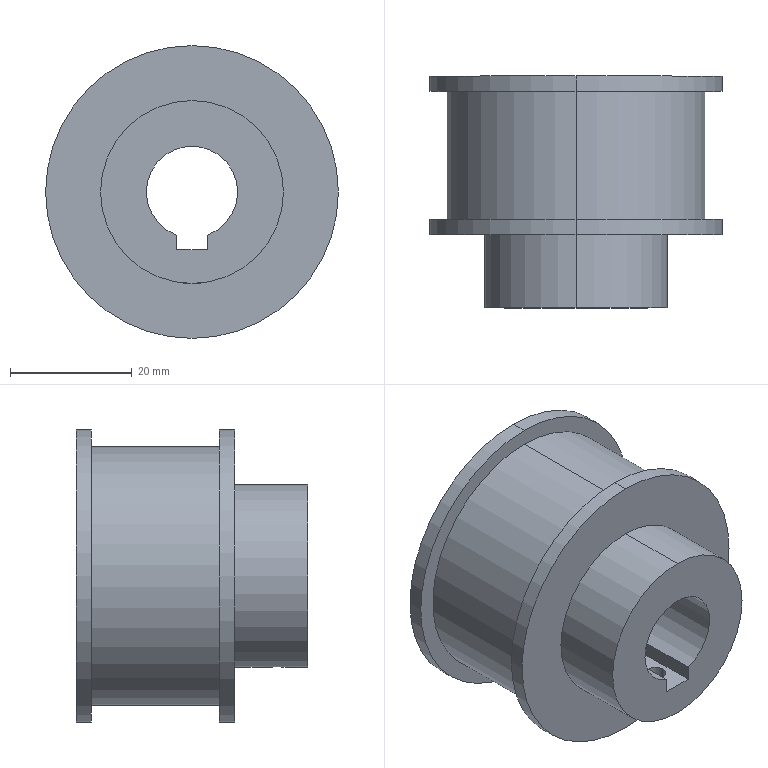Part | STEP file | PN_0026 (ATP14L075)_ATP22XL050-A-H8 | 1 solid | 19 faces | box 48 x 38 x 48 mm | volume 40082 mm3 | cylinder 11 | plane 8 | commonest cylinder face diameters 48 x4 3.3 x2 30 x2 42.45 x2 15 x1